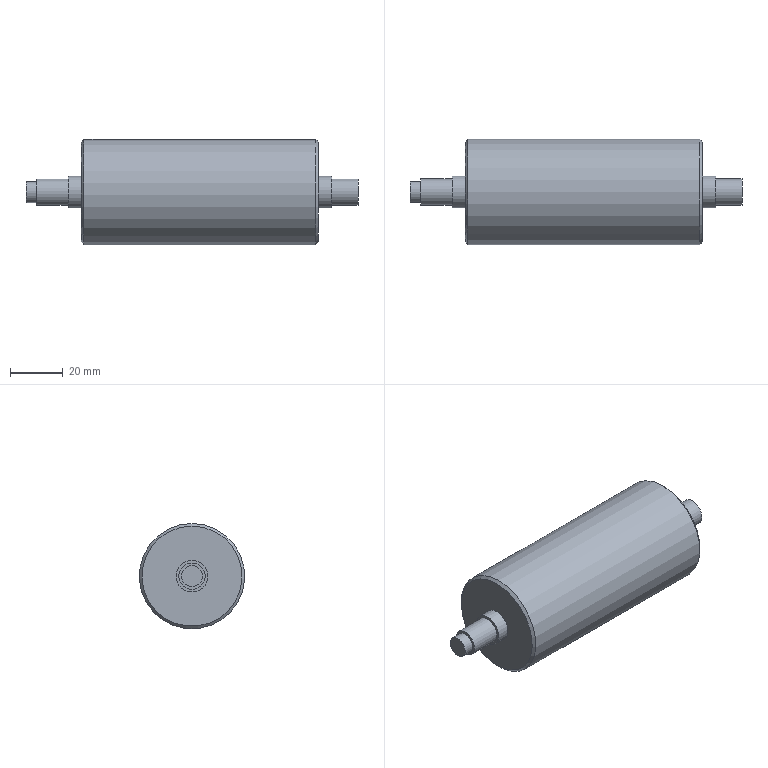Part | NX | features DATUM_CSYS 2, SKETCH 1, SWP104 1 | 1 solid | 15 faces | box 126 x 40 x 40 mm | volume 116034 mm3 | plane 7 | cylinder 6 | cone 2 | commonest cylinder face diameters 10 x2 12 x2 8 x1 40 x1
STEP:
#1=CARTESIAN_POINT('',(-66.,0.,4.));
#2=VERTEX_POINT('',#1);
#3=CARTESIAN_POINT('',(-66.,0.,0.));
#4=DIRECTION('',(-1.,0.,0.));
#5=DIRECTION('',(0.,0.,1.));
#6=AXIS2_PLACEMENT_3D('',#3,#4,#5);
#7=CIRCLE('',#6,4.);
#8=EDGE_CURVE('',#2,#2,#7,.T.);
#9=ORIENTED_EDGE('',*,*,#8,.T.);
#10=EDGE_LOOP('',(#9));
#11=FACE_BOUND('',#10,.T.);
#12=CARTESIAN_POINT('',(-66.,4.,0.));
#13=DIRECTION('',(1.,0.,0.));
#14=DIRECTION('',(0.,0.,-1.));
#15=AXIS2_PLACEMENT_3D('',#12,#13,#14);
#16=PLANE('',#15);
#17=ADVANCED_FACE('',(#11),#16,.F.);
#18=CARTESIAN_POINT('',(60.,0.,5.));
#19=VERTEX_POINT('',#18);
#20=CARTESIAN_POINT('',(60.,0.,0.));
#21=DIRECTION('',(-1.,0.,0.));
#22=DIRECTION('',(0.,0.,1.));
#23=AXIS2_PLACEMENT_3D('',#20,#21,#22);
#24=CIRCLE('',#23,5.);
#25=EDGE_CURVE('',#19,#19,#24,.T.);
#26=ORIENTED_EDGE('',*,*,#25,.F.);
#27=EDGE_LOOP('',(#26));
#28=FACE_BOUND('',#27,.T.);
#29=CARTESIAN_POINT('',(60.,0.,0.));
#30=DIRECTION('',(-1.,0.,0.));
#31=DIRECTION('',(0.,0.,1.));
#32=AXIS2_PLACEMENT_3D('',#29,#30,#31);
#33=PLANE('',#32);
#34=ADVANCED_FACE('',(#28),#33,.F.);
#35=CARTESIAN_POINT('',(50.,0.,5.));
#36=VERTEX_POINT('',#35);
#37=CARTESIAN_POINT('',(50.,0.,0.));
#38=DIRECTION('',(-1.,0.,0.));
#39=DIRECTION('',(0.,0.,1.));
#40=AXIS2_PLACEMENT_3D('',#37,#38,#39);
#41=CIRCLE('',#40,5.);
#42=EDGE_CURVE('',#36,#36,#41,.T.);
#43=ORIENTED_EDGE('',*,*,#42,.F.);
#44=EDGE_LOOP('',(#43));
#45=FACE_BOUND('',#44,.T.);
#46=ORIENTED_EDGE('',*,*,#25,.T.);
#47=EDGE_LOOP('',(#46));
#48=FACE_BOUND('',#47,.T.);
#49=CARTESIAN_POINT('',(60.,0.,0.));
#50=DIRECTION('',(-1.,0.,0.));
#51=DIRECTION('',(0.,0.,1.));
#52=AXIS2_PLACEMENT_3D('',#49,#50,#51);
#53=CYLINDRICAL_SURFACE('',#52,5.);
#54=ADVANCED_FACE('',(#45,#48),#53,.T.);
#55=CARTESIAN_POINT('',(50.,0.,6.));
#56=VERTEX_POINT('',#55);
#57=CARTESIAN_POINT('',(50.,0.,0.));
#58=DIRECTION('',(-1.,0.,0.));
#59=DIRECTION('',(0.,0.,1.));
#60=AXIS2_PLACEMENT_3D('',#57,#58,#59);
#61=CIRCLE('',#60,6.);
#62=EDGE_CURVE('',#56,#56,#61,.T.);
#63=ORIENTED_EDGE('',*,*,#62,.F.);
#64=EDGE_LOOP('',(#63));
#65=FACE_BOUND('',#64,.T.);
#66=ORIENTED_EDGE('',*,*,#42,.T.);
#67=EDGE_LOOP('',(#66));
#68=FACE_BOUND('',#67,.T.);
#69=CARTESIAN_POINT('',(50.,5.,0.));
#70=DIRECTION('',(-1.,0.,0.));
#71=DIRECTION('',(0.,0.,1.));
#72=AXIS2_PLACEMENT_3D('',#69,#70,#71);
#73=PLANE('',#72);
#74=ADVANCED_FACE('',(#65,#68),#73,.F.);
#75=CARTESIAN_POINT('',(45.,0.,6.));
#76=VERTEX_POINT('',#75);
#77=CARTESIAN_POINT('',(45.,0.,0.));
#78=DIRECTION('',(-1.,0.,0.));
#79=DIRECTION('',(0.,0.,1.));
#80=AXIS2_PLACEMENT_3D('',#77,#78,#79);
#81=CIRCLE('',#80,6.);
#82=EDGE_CURVE('',#76,#76,#81,.T.);
#83=ORIENTED_EDGE('',*,*,#82,.F.);
#84=EDGE_LOOP('',(#83));
#85=FACE_BOUND('',#84,.T.);
#86=ORIENTED_EDGE('',*,*,#62,.T.);
#87=EDGE_LOOP('',(#86));
#88=FACE_BOUND('',#87,.T.);
#89=CARTESIAN_POINT('',(60.,0.,0.));
#90=DIRECTION('',(-1.,0.,0.));
#91=DIRECTION('',(0.,0.,1.));
#92=AXIS2_PLACEMENT_3D('',#89,#90,#91);
#93=CYLINDRICAL_SURFACE('',#92,6.);
#94=ADVANCED_FACE('',(#85,#88),#93,.T.);
#95=CARTESIAN_POINT('',(45.,0.,19.));
#96=VERTEX_POINT('',#95);
#97=CARTESIAN_POINT('',(45.,0.,0.));
#98=DIRECTION('',(-1.,0.,0.));
#99=DIRECTION('',(0.,0.,1.));
#100=AXIS2_PLACEMENT_3D('',#97,#98,#99);
#101=CIRCLE('',#100,19.);
#102=EDGE_CURVE('',#96,#96,#101,.T.);
#103=ORIENTED_EDGE('',*,*,#102,.F.);
#104=EDGE_LOOP('',(#103));
#105=FACE_BOUND('',#104,.T.);
#106=ORIENTED_EDGE('',*,*,#82,.T.);
#107=EDGE_LOOP('',(#106));
#108=FACE_BOUND('',#107,.T.);
#109=CARTESIAN_POINT('',(45.,6.,0.));
#110=DIRECTION('',(-1.,0.,0.));
#111=DIRECTION('',(0.,0.,1.));
#112=AXIS2_PLACEMENT_3D('',#109,#110,#111);
#113=PLANE('',#112);
#114=ADVANCED_FACE('',(#105,#108),#113,.F.);
#115=CARTESIAN_POINT('',(44.,0.,20.));
#116=VERTEX_POINT('',#115);
#117=CARTESIAN_POINT('',(44.,0.,0.));
#118=DIRECTION('',(-1.,0.,0.));
#119=DIRECTION('',(0.,0.,1.));
#120=AXIS2_PLACEMENT_3D('',#117,#118,#119);
#121=CIRCLE('',#120,20.);
#122=EDGE_CURVE('',#116,#116,#121,.T.);
#123=ORIENTED_EDGE('',*,*,#122,.F.);
#124=EDGE_LOOP('',(#123));
#125=FACE_BOUND('',#124,.T.);
#126=ORIENTED_EDGE('',*,*,#102,.T.);
#127=EDGE_LOOP('',(#126));
#128=FACE_BOUND('',#127,.T.);
#129=CARTESIAN_POINT('',(45.,0.,0.));
#130=DIRECTION('',(-1.,0.,0.));
#131=DIRECTION('',(0.,0.,1.));
#132=AXIS2_PLACEMENT_3D('',#129,#130,#131);
#133=CONICAL_SURFACE('',#132,19.,0.7854);
#134=ADVANCED_FACE('',(#125,#128),#133,.T.);
#135=CARTESIAN_POINT('',(-44.,0.,20.));
#136=VERTEX_POINT('',#135);
#137=CARTESIAN_POINT('',(-44.,0.,0.));
#138=DIRECTION('',(-1.,0.,0.));
#139=DIRECTION('',(0.,0.,1.));
#140=AXIS2_PLACEMENT_3D('',#137,#138,#139);
#141=CIRCLE('',#140,20.);
#142=EDGE_CURVE('',#136,#136,#141,.T.);
#143=ORIENTED_EDGE('',*,*,#142,.F.);
#144=EDGE_LOOP('',(#143));
#145=FACE_BOUND('',#144,.T.);
#146=ORIENTED_EDGE('',*,*,#122,.T.);
#147=EDGE_LOOP('',(#146));
#148=FACE_BOUND('',#147,.T.);
#149=CARTESIAN_POINT('',(60.,0.,0.));
#150=DIRECTION('',(-1.,0.,0.));
#151=DIRECTION('',(0.,0.,1.));
#152=AXIS2_PLACEMENT_3D('',#149,#150,#151);
#153=CYLINDRICAL_SURFACE('',#152,20.);
#154=ADVANCED_FACE('',(#145,#148),#153,.T.);
#155=CARTESIAN_POINT('',(-45.,0.,19.));
#156=VERTEX_POINT('',#155);
#157=CARTESIAN_POINT('',(-45.,0.,0.));
#158=DIRECTION('',(-1.,0.,0.));
#159=DIRECTION('',(0.,0.,1.));
#160=AXIS2_PLACEMENT_3D('',#157,#158,#159);
#161=CIRCLE('',#160,19.);
#162=EDGE_CURVE('',#156,#156,#161,.T.);
#163=ORIENTED_EDGE('',*,*,#162,.F.);
#164=EDGE_LOOP('',(#163));
#165=FACE_BOUND('',#164,.T.);
#166=ORIENTED_EDGE('',*,*,#142,.T.);
#167=EDGE_LOOP('',(#166));
#168=FACE_BOUND('',#167,.T.);
#169=CARTESIAN_POINT('',(-44.,0.,0.));
#170=DIRECTION('',(1.,0.,0.));
#171=DIRECTION('',(0.,0.,-1.));
#172=AXIS2_PLACEMENT_3D('',#169,#170,#171);
#173=CONICAL_SURFACE('',#172,20.,0.7854);
#174=ADVANCED_FACE('',(#165,#168),#173,.T.);
#175=CARTESIAN_POINT('',(-45.,0.,6.));
#176=VERTEX_POINT('',#175);
#177=CARTESIAN_POINT('',(-45.,0.,0.));
#178=DIRECTION('',(-1.,0.,0.));
#179=DIRECTION('',(0.,0.,1.));
#180=AXIS2_PLACEMENT_3D('',#177,#178,#179);
#181=CIRCLE('',#180,6.);
#182=EDGE_CURVE('',#176,#176,#181,.T.);
#183=ORIENTED_EDGE('',*,*,#182,.F.);
#184=EDGE_LOOP('',(#183));
#185=FACE_BOUND('',#184,.T.);
#186=ORIENTED_EDGE('',*,*,#162,.T.);
#187=EDGE_LOOP('',(#186));
#188=FACE_BOUND('',#187,.T.);
#189=CARTESIAN_POINT('',(-45.,19.,0.));
#190=DIRECTION('',(1.,0.,0.));
#191=DIRECTION('',(0.,0.,-1.));
#192=AXIS2_PLACEMENT_3D('',#189,#190,#191);
#193=PLANE('',#192);
#194=ADVANCED_FACE('',(#185,#188),#193,.F.);
#195=CARTESIAN_POINT('',(-50.,0.,6.));
#196=VERTEX_POINT('',#195);
#197=CARTESIAN_POINT('',(-50.,0.,0.));
#198=DIRECTION('',(-1.,0.,0.));
#199=DIRECTION('',(0.,0.,1.));
#200=AXIS2_PLACEMENT_3D('',#197,#198,#199);
#201=CIRCLE('',#200,6.);
#202=EDGE_CURVE('',#196,#196,#201,.T.);
#203=ORIENTED_EDGE('',*,*,#202,.F.);
#204=EDGE_LOOP('',(#203));
#205=FACE_BOUND('',#204,.T.);
#206=ORIENTED_EDGE('',*,*,#182,.T.);
#207=EDGE_LOOP('',(#206));
#208=FACE_BOUND('',#207,.T.);
#209=CARTESIAN_POINT('',(60.,0.,0.));
#210=DIRECTION('',(-1.,0.,0.));
#211=DIRECTION('',(0.,0.,1.));
#212=AXIS2_PLACEMENT_3D('',#209,#210,#211);
#213=CYLINDRICAL_SURFACE('',#212,6.);
#214=ADVANCED_FACE('',(#205,#208),#213,.T.);
#215=CARTESIAN_POINT('',(-50.,0.,5.));
#216=VERTEX_POINT('',#215);
#217=CARTESIAN_POINT('',(-50.,0.,0.));
#218=DIRECTION('',(-1.,0.,0.));
#219=DIRECTION('',(0.,0.,1.));
#220=AXIS2_PLACEMENT_3D('',#217,#218,#219);
#221=CIRCLE('',#220,5.);
#222=EDGE_CURVE('',#216,#216,#221,.T.);
#223=ORIENTED_EDGE('',*,*,#222,.F.);
#224=EDGE_LOOP('',(#223));
#225=FACE_BOUND('',#224,.T.);
#226=ORIENTED_EDGE('',*,*,#202,.T.);
#227=EDGE_LOOP('',(#226));
#228=FACE_BOUND('',#227,.T.);
#229=CARTESIAN_POINT('',(-50.,6.,0.));
#230=DIRECTION('',(1.,0.,0.));
#231=DIRECTION('',(0.,0.,-1.));
#232=AXIS2_PLACEMENT_3D('',#229,#230,#231);
#233=PLANE('',#232);
#234=ADVANCED_FACE('',(#225,#228),#233,.F.);
#235=CARTESIAN_POINT('',(-62.,0.,5.));
#236=VERTEX_POINT('',#235);
#237=CARTESIAN_POINT('',(-62.,0.,0.));
#238=DIRECTION('',(-1.,0.,0.));
#239=DIRECTION('',(0.,0.,1.));
#240=AXIS2_PLACEMENT_3D('',#237,#238,#239);
#241=CIRCLE('',#240,5.);
#242=EDGE_CURVE('',#236,#236,#241,.T.);
#243=ORIENTED_EDGE('',*,*,#242,.F.);
#244=EDGE_LOOP('',(#243));
#245=FACE_BOUND('',#244,.T.);
#246=ORIENTED_EDGE('',*,*,#222,.T.);
#247=EDGE_LOOP('',(#246));
#248=FACE_BOUND('',#247,.T.);
#249=CARTESIAN_POINT('',(60.,0.,0.));
#250=DIRECTION('',(-1.,0.,0.));
#251=DIRECTION('',(0.,0.,1.));
#252=AXIS2_PLACEMENT_3D('',#249,#250,#251);
#253=CYLINDRICAL_SURFACE('',#252,5.);
#254=ADVANCED_FACE('',(#245,#248),#253,.T.);
#255=CARTESIAN_POINT('',(-62.,0.,4.));
#256=VERTEX_POINT('',#255);
#257=CARTESIAN_POINT('',(-62.,0.,0.));
#258=DIRECTION('',(-1.,0.,0.));
#259=DIRECTION('',(0.,0.,1.));
#260=AXIS2_PLACEMENT_3D('',#257,#258,#259);
#261=CIRCLE('',#260,4.);
#262=EDGE_CURVE('',#256,#256,#261,.T.);
#263=ORIENTED_EDGE('',*,*,#262,.F.);
#264=EDGE_LOOP('',(#263));
#265=FACE_BOUND('',#264,.T.);
#266=ORIENTED_EDGE('',*,*,#242,.T.);
#267=EDGE_LOOP('',(#266));
#268=FACE_BOUND('',#267,.T.);
#269=CARTESIAN_POINT('',(-62.,5.,0.));
#270=DIRECTION('',(1.,0.,0.));
#271=DIRECTION('',(0.,0.,-1.));
#272=AXIS2_PLACEMENT_3D('',#269,#270,#271);
#273=PLANE('',#272);
#274=ADVANCED_FACE('',(#265,#268),#273,.F.);
#275=ORIENTED_EDGE('',*,*,#8,.F.);
#276=EDGE_LOOP('',(#275));
#277=FACE_BOUND('',#276,.T.);
#278=ORIENTED_EDGE('',*,*,#262,.T.);
#279=EDGE_LOOP('',(#278));
#280=FACE_BOUND('',#279,.T.);
#281=CARTESIAN_POINT('',(60.,0.,0.));
#282=DIRECTION('',(-1.,0.,0.));
#283=DIRECTION('',(0.,0.,1.));
#284=AXIS2_PLACEMENT_3D('',#281,#282,#283);
#285=CYLINDRICAL_SURFACE('',#284,4.);
#286=ADVANCED_FACE('',(#277,#280),#285,.T.);
#287=CLOSED_SHELL('',(#17,#34,#54,#74,#94,#114,#134,#154,#174,#194,#214,#234,#254,#274,#286));
#288=MANIFOLD_SOLID_BREP('',#287);
#289=(LENGTH_UNIT()NAMED_UNIT(*)SI_UNIT(.MILLI.,.METRE.));
#290=UNCERTAINTY_MEASURE_WITH_UNIT(LENGTH_MEASURE(0.00001),#289,'','');
#291=(NAMED_UNIT(*)PLANE_ANGLE_UNIT()SI_UNIT($,.RADIAN.));
#292=(NAMED_UNIT(*)SI_UNIT($,.STERADIAN.)SOLID_ANGLE_UNIT());
#293=(GEOMETRIC_REPRESENTATION_CONTEXT(3)GLOBAL_UNCERTAINTY_ASSIGNED_CONTEXT((#290))GLOBAL_UNIT_ASSIGNED_CONTEXT((#289,#291,#292))REPRESENTATION_CONTEXT('',''));
#294=ADVANCED_BREP_SHAPE_REPRESENTATION('',(#288),#293);